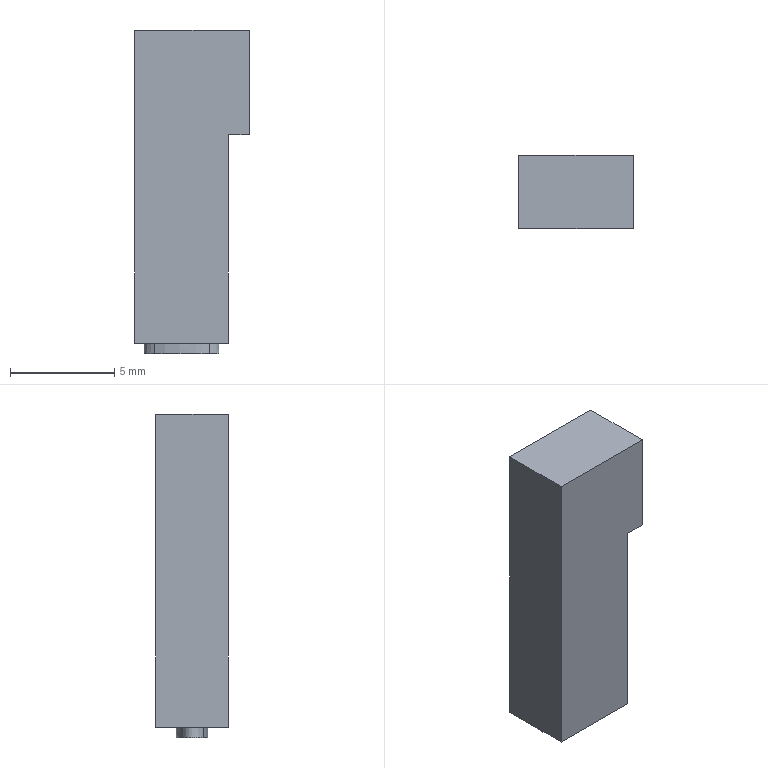Part | STEP file | gslz 2016.10.28-10_id1658_x_t | 1 solid | 15 faces | box 5.5 x 3.5 x 15.5 mm | volume 254.67 mm3 | plane 10 | other 5
STEP:
#1=CARTESIAN_POINT('',(0.,0.,0.));
#2=DIRECTION('',(0.,0.,1.));
#3=DIRECTION('',(1.,0.,0.));
#4=AXIS2_PLACEMENT_3D('',#1,#2,#3);
#5=CARTESIAN_POINT('',(-690.499,76.038,0.));
#6=VERTEX_POINT('',#5);
#7=CARTESIAN_POINT('',(-693.11,74.96,0.));
#8=VERTEX_POINT('',#7);
#9=CARTESIAN_POINT('',(-690.499,76.038,0.));
#10=CARTESIAN_POINT('',(-690.821,76.179,0.));
#11=CARTESIAN_POINT('',(-691.26,76.249,0.));
#12=CARTESIAN_POINT('',(-692.38,76.249,0.));
#13=CARTESIAN_POINT('',(-692.816,76.179,0.));
#14=CARTESIAN_POINT('',(-693.444,75.897,0.));
#15=CARTESIAN_POINT('',(-693.601,75.72,0.));
#16=CARTESIAN_POINT('',(-693.601,75.283,0.));
#17=CARTESIAN_POINT('',(-693.437,75.101,0.));
#18=CARTESIAN_POINT('',(-693.11,74.96,0.));
#19=B_SPLINE_CURVE_WITH_KNOTS('',3,(#9,#10,#11,#12,#13,#14,#15,#16,#17,#18),.UNSPECIFIED.,.F.,.F.,(4,2,2,2,4),(0.,0.2476,0.4947,0.7418,1.),.UNSPECIFIED.);
#20=CARTESIAN_POINT('',(-694.06,75.499,0.));
#21=DIRECTION('',(0.,0.,1.));
#22=DIRECTION('',(1.,0.,0.));
#23=AXIS2_PLACEMENT_3D('',#20,#21,#22);
#24=PLANE('',#23);
#25=CARTESIAN_POINT('',(3.561,0.539));
#26=CARTESIAN_POINT('',(3.239,0.6797));
#27=CARTESIAN_POINT('',(2.8,0.75));
#28=CARTESIAN_POINT('',(1.68,0.75));
#29=CARTESIAN_POINT('',(1.244,0.6797));
#30=CARTESIAN_POINT('',(0.6161,0.3984));
#31=CARTESIAN_POINT('',(0.4587,0.2209));
#32=CARTESIAN_POINT('',(0.4587,-0.2161));
#33=CARTESIAN_POINT('',(0.6228,-0.3977));
#34=CARTESIAN_POINT('',(0.95,-0.539));
#35=B_SPLINE_CURVE_WITH_KNOTS('',3,(#25,#26,#27,#28,#29,#30,#31,#32,#33,#34),.UNSPECIFIED.,.F.,.F.,(4,2,2,2,4),(0.,0.2476,0.4947,0.7418,1.),.UNSPECIFIED.);
#36=(GEOMETRIC_REPRESENTATION_CONTEXT(2)PARAMETRIC_REPRESENTATION_CONTEXT()REPRESENTATION_CONTEXT('',''));
#37=DEFINITIONAL_REPRESENTATION('',(#35),#36);
#38=PCURVE('',#24,#37);
#39=CARTESIAN_POINT('',(-693.11,74.96,-0.5));
#40=CARTESIAN_POINT('',(-693.437,75.101,-0.5));
#41=CARTESIAN_POINT('',(-693.601,75.283,-0.5));
#42=CARTESIAN_POINT('',(-693.601,75.72,-0.5));
#43=CARTESIAN_POINT('',(-693.444,75.897,-0.5));
#44=CARTESIAN_POINT('',(-692.816,76.179,-0.5));
#45=CARTESIAN_POINT('',(-692.38,76.249,-0.5));
#46=CARTESIAN_POINT('',(-691.26,76.249,-0.5));
#47=CARTESIAN_POINT('',(-690.821,76.179,-0.5));
#48=CARTESIAN_POINT('',(-690.499,76.038,-0.5));
#49=B_SPLINE_CURVE_WITH_KNOTS('',3,(#39,#40,#41,#42,#43,#44,#45,#46,#47,#48),.UNSPECIFIED.,.F.,.F.,(4,2,2,2,4),(0.,0.2582,0.5053,0.7524,1.),.UNSPECIFIED.);
#50=DIRECTION('',(0.,0.,1.));
#51=VECTOR('',#50,1.);
#52=SURFACE_OF_LINEAR_EXTRUSION('',#49,#51);
#53=CARTESIAN_POINT('',(1.,0.5));
#54=DIRECTION('',(-1.,0.));
#55=VECTOR('',#54,1.);
#56=LINE('',#53,#55);
#57=(GEOMETRIC_REPRESENTATION_CONTEXT(2)PARAMETRIC_REPRESENTATION_CONTEXT()REPRESENTATION_CONTEXT('',''));
#58=DEFINITIONAL_REPRESENTATION('',(#56),#57);
#59=PCURVE('',#52,#58);
#60=SURFACE_CURVE('',#19,(#38,#59),.PCURVE_S1.);
#61=EDGE_CURVE('',#6,#8,#60,.T.);
#62=ORIENTED_EDGE('',*,*,#61,.T.);
#63=CARTESIAN_POINT('',(-690.49,74.967,0.));
#64=VERTEX_POINT('',#63);
#65=CARTESIAN_POINT('',(-693.11,74.96,0.));
#66=CARTESIAN_POINT('',(-692.782,74.819,0.));
#67=CARTESIAN_POINT('',(-692.352,74.749,0.));
#68=CARTESIAN_POINT('',(-691.247,74.749,0.));
#69=CARTESIAN_POINT('',(-690.804,74.822,0.));
#70=CARTESIAN_POINT('',(-690.49,74.967,0.));
#71=B_SPLINE_CURVE_WITH_KNOTS('',3,(#65,#66,#67,#68,#69,#70),.UNSPECIFIED.,.F.,.F.,(4,2,4),(0.,0.4809,1.),.UNSPECIFIED.);
#72=CARTESIAN_POINT('',(0.95,-0.539));
#73=CARTESIAN_POINT('',(1.278,-0.6797));
#74=CARTESIAN_POINT('',(1.708,-0.75));
#75=CARTESIAN_POINT('',(2.813,-0.75));
#76=CARTESIAN_POINT('',(3.256,-0.6769));
#77=CARTESIAN_POINT('',(3.57,-0.5315));
#78=B_SPLINE_CURVE_WITH_KNOTS('',3,(#72,#73,#74,#75,#76,#77),.UNSPECIFIED.,.F.,.F.,(4,2,4),(0.,0.4809,1.),.UNSPECIFIED.);
#79=(GEOMETRIC_REPRESENTATION_CONTEXT(2)PARAMETRIC_REPRESENTATION_CONTEXT()REPRESENTATION_CONTEXT('',''));
#80=DEFINITIONAL_REPRESENTATION('',(#78),#79);
#81=PCURVE('',#24,#80);
#82=CARTESIAN_POINT('',(-690.49,74.967,-0.5));
#83=CARTESIAN_POINT('',(-690.804,74.822,-0.5));
#84=CARTESIAN_POINT('',(-691.247,74.749,-0.5));
#85=CARTESIAN_POINT('',(-692.352,74.749,-0.5));
#86=CARTESIAN_POINT('',(-692.782,74.819,-0.5));
#87=CARTESIAN_POINT('',(-693.11,74.96,-0.5));
#88=B_SPLINE_CURVE_WITH_KNOTS('',3,(#82,#83,#84,#85,#86,#87),.UNSPECIFIED.,.F.,.F.,(4,2,4),(0.,0.5191,1.),.UNSPECIFIED.);
#89=DIRECTION('',(0.,0.,1.));
#90=VECTOR('',#89,1.);
#91=SURFACE_OF_LINEAR_EXTRUSION('',#88,#90);
#92=CARTESIAN_POINT('',(1.,0.5));
#93=DIRECTION('',(-1.,0.));
#94=VECTOR('',#93,1.);
#95=LINE('',#92,#94);
#96=(GEOMETRIC_REPRESENTATION_CONTEXT(2)PARAMETRIC_REPRESENTATION_CONTEXT()REPRESENTATION_CONTEXT('',''));
#97=DEFINITIONAL_REPRESENTATION('',(#95),#96);
#98=PCURVE('',#91,#97);
#99=SURFACE_CURVE('',#71,(#81,#98),.PCURVE_S1.);
#100=EDGE_CURVE('',#8,#64,#99,.T.);
#101=ORIENTED_EDGE('',*,*,#100,.T.);
#102=CARTESIAN_POINT('',(-690.49,74.967,0.));
#103=CARTESIAN_POINT('',(-690.175,75.113,0.));
#104=CARTESIAN_POINT('',(-690.019,75.292,0.));
#105=CARTESIAN_POINT('',(-690.019,75.72,0.));
#106=CARTESIAN_POINT('',(-690.179,75.897,0.));
#107=CARTESIAN_POINT('',(-690.499,76.038,0.));
#108=B_SPLINE_CURVE_WITH_KNOTS('',3,(#102,#103,#104,#105,#106,#107),.UNSPECIFIED.,.F.,.F.,(4,2,4),(0.,0.5,1.),.UNSPECIFIED.);
#109=CARTESIAN_POINT('',(3.57,-0.5315));
#110=CARTESIAN_POINT('',(3.885,-0.3861));
#111=CARTESIAN_POINT('',(4.041,-0.2065));
#112=CARTESIAN_POINT('',(4.041,0.2209));
#113=CARTESIAN_POINT('',(3.881,0.3984));
#114=CARTESIAN_POINT('',(3.561,0.539));
#115=B_SPLINE_CURVE_WITH_KNOTS('',3,(#109,#110,#111,#112,#113,#114),.UNSPECIFIED.,.F.,.F.,(4,2,4),(0.,0.5,1.),.UNSPECIFIED.);
#116=(GEOMETRIC_REPRESENTATION_CONTEXT(2)PARAMETRIC_REPRESENTATION_CONTEXT()REPRESENTATION_CONTEXT('',''));
#117=DEFINITIONAL_REPRESENTATION('',(#115),#116);
#118=PCURVE('',#24,#117);
#119=CARTESIAN_POINT('',(-690.499,76.038,-0.5));
#120=CARTESIAN_POINT('',(-690.179,75.897,-0.5));
#121=CARTESIAN_POINT('',(-690.019,75.72,-0.5));
#122=CARTESIAN_POINT('',(-690.019,75.292,-0.5));
#123=CARTESIAN_POINT('',(-690.175,75.113,-0.5));
#124=CARTESIAN_POINT('',(-690.49,74.967,-0.5));
#125=B_SPLINE_CURVE_WITH_KNOTS('',3,(#119,#120,#121,#122,#123,#124),.UNSPECIFIED.,.F.,.F.,(4,2,4),(0.,0.5,1.),.UNSPECIFIED.);
#126=DIRECTION('',(0.,0.,1.));
#127=VECTOR('',#126,1.);
#128=SURFACE_OF_LINEAR_EXTRUSION('',#125,#127);
#129=CARTESIAN_POINT('',(1.,0.5));
#130=DIRECTION('',(-1.,0.));
#131=VECTOR('',#130,1.);
#132=LINE('',#129,#131);
#133=(GEOMETRIC_REPRESENTATION_CONTEXT(2)PARAMETRIC_REPRESENTATION_CONTEXT()REPRESENTATION_CONTEXT('',''));
#134=DEFINITIONAL_REPRESENTATION('',(#132),#133);
#135=PCURVE('',#128,#134);
#136=SURFACE_CURVE('',#108,(#118,#135),.PCURVE_S1.);
#137=EDGE_CURVE('',#64,#6,#136,.T.);
#138=ORIENTED_EDGE('',*,*,#137,.T.);
#139=EDGE_LOOP('',(#62,#101,#138));
#140=FACE_BOUND('',#139,.T.);
#141=CARTESIAN_POINT('',(-689.56,77.249,0.));
#142=VERTEX_POINT('',#141);
#143=CARTESIAN_POINT('',(-689.56,73.749,0.));
#144=VERTEX_POINT('',#143);
#145=CARTESIAN_POINT('',(-689.56,75.499,0.));
#146=DIRECTION('',(0.,-1.,0.));
#147=VECTOR('',#146,1.);
#148=LINE('',#145,#147);
#149=CARTESIAN_POINT('',(4.5,0.));
#150=DIRECTION('',(0.,-1.));
#151=VECTOR('',#150,1.);
#152=LINE('',#149,#151);
#153=(GEOMETRIC_REPRESENTATION_CONTEXT(2)PARAMETRIC_REPRESENTATION_CONTEXT()REPRESENTATION_CONTEXT('',''));
#154=DEFINITIONAL_REPRESENTATION('',(#152),#153);
#155=PCURVE('',#24,#154);
#156=CARTESIAN_POINT('',(-689.56,75.499,7.5));
#157=DIRECTION('',(1.,0.,0.));
#158=DIRECTION('',(0.,0.,-1.));
#159=AXIS2_PLACEMENT_3D('',#156,#157,#158);
#160=PLANE('',#159);
#161=CARTESIAN_POINT('',(7.5,0.000000303));
#162=DIRECTION('',(0.,-1.));
#163=VECTOR('',#162,1.);
#164=LINE('',#161,#163);
#165=(GEOMETRIC_REPRESENTATION_CONTEXT(2)PARAMETRIC_REPRESENTATION_CONTEXT()REPRESENTATION_CONTEXT('',''));
#166=DEFINITIONAL_REPRESENTATION('',(#164),#165);
#167=PCURVE('',#160,#166);
#168=SURFACE_CURVE('',#148,(#155,#167),.PCURVE_S1.);
#169=EDGE_CURVE('',#142,#144,#168,.T.);
#170=ORIENTED_EDGE('',*,*,#169,.T.);
#171=CARTESIAN_POINT('',(-694.06,73.749,0.));
#172=VERTEX_POINT('',#171);
#173=CARTESIAN_POINT('',(-691.31,73.749,0.));
#174=DIRECTION('',(-1.,0.000000055,0.));
#175=VECTOR('',#174,1.);
#176=LINE('',#173,#175);
#177=CARTESIAN_POINT('',(2.75,-1.75));
#178=DIRECTION('',(-1.,0.000000055));
#179=VECTOR('',#178,1.);
#180=LINE('',#177,#179);
#181=(GEOMETRIC_REPRESENTATION_CONTEXT(2)PARAMETRIC_REPRESENTATION_CONTEXT()REPRESENTATION_CONTEXT('',''));
#182=DEFINITIONAL_REPRESENTATION('',(#180),#181);
#183=PCURVE('',#24,#182);
#184=CARTESIAN_POINT('',(-694.06,73.749,15.));
#185=DIRECTION('',(-0.000000055,-1.,0.));
#186=DIRECTION('',(-1.,0.000000055,0.));
#187=AXIS2_PLACEMENT_3D('',#184,#185,#186);
#188=PLANE('',#187);
#189=CARTESIAN_POINT('',(-2.75,15.));
#190=DIRECTION('',(1.,0.));
#191=VECTOR('',#190,1.);
#192=LINE('',#189,#191);
#193=(GEOMETRIC_REPRESENTATION_CONTEXT(2)PARAMETRIC_REPRESENTATION_CONTEXT()REPRESENTATION_CONTEXT('',''));
#194=DEFINITIONAL_REPRESENTATION('',(#192),#193);
#195=PCURVE('',#188,#194);
#196=SURFACE_CURVE('',#176,(#183,#195),.PCURVE_S1.);
#197=EDGE_CURVE('',#144,#172,#196,.T.);
#198=ORIENTED_EDGE('',*,*,#197,.T.);
#199=CARTESIAN_POINT('',(-694.06,77.249,0.));
#200=VERTEX_POINT('',#199);
#201=CARTESIAN_POINT('',(-694.06,75.499,0.));
#202=DIRECTION('',(0.,1.,0.));
#203=VECTOR('',#202,1.);
#204=LINE('',#201,#203);
#205=CARTESIAN_POINT('',(0.,0.));
#206=DIRECTION('',(0.,1.));
#207=VECTOR('',#206,1.);
#208=LINE('',#205,#207);
#209=(GEOMETRIC_REPRESENTATION_CONTEXT(2)PARAMETRIC_REPRESENTATION_CONTEXT()REPRESENTATION_CONTEXT('',''));
#210=DEFINITIONAL_REPRESENTATION('',(#208),#209);
#211=PCURVE('',#24,#210);
#212=CARTESIAN_POINT('',(-694.06,77.249,15.));
#213=DIRECTION('',(-1.,0.,0.));
#214=DIRECTION('',(0.,1.,0.));
#215=AXIS2_PLACEMENT_3D('',#212,#213,#214);
#216=PLANE('',#215);
#217=CARTESIAN_POINT('',(-1.75,15.));
#218=DIRECTION('',(1.,0.));
#219=VECTOR('',#218,1.);
#220=LINE('',#217,#219);
#221=(GEOMETRIC_REPRESENTATION_CONTEXT(2)PARAMETRIC_REPRESENTATION_CONTEXT()REPRESENTATION_CONTEXT('',''));
#222=DEFINITIONAL_REPRESENTATION('',(#220),#221);
#223=PCURVE('',#216,#222);
#224=SURFACE_CURVE('',#204,(#211,#223),.PCURVE_S1.);
#225=EDGE_CURVE('',#172,#200,#224,.T.);
#226=ORIENTED_EDGE('',*,*,#225,.T.);
#227=CARTESIAN_POINT('',(-691.31,77.249,0.));
#228=DIRECTION('',(1.,-0.000000055,0.));
#229=VECTOR('',#228,1.);
#230=LINE('',#227,#229);
#231=CARTESIAN_POINT('',(2.75,1.75));
#232=DIRECTION('',(1.,-0.000000055));
#233=VECTOR('',#232,1.);
#234=LINE('',#231,#233);
#235=(GEOMETRIC_REPRESENTATION_CONTEXT(2)PARAMETRIC_REPRESENTATION_CONTEXT()REPRESENTATION_CONTEXT('',''));
#236=DEFINITIONAL_REPRESENTATION('',(#234),#235);
#237=PCURVE('',#24,#236);
#238=CARTESIAN_POINT('',(-688.56,77.249,15.));
#239=DIRECTION('',(0.000000055,1.,0.));
#240=DIRECTION('',(1.,-0.000000055,0.));
#241=AXIS2_PLACEMENT_3D('',#238,#239,#240);
#242=PLANE('',#241);
#243=CARTESIAN_POINT('',(-2.75,15.));
#244=DIRECTION('',(1.,0.));
#245=VECTOR('',#244,1.);
#246=LINE('',#243,#245);
#247=(GEOMETRIC_REPRESENTATION_CONTEXT(2)PARAMETRIC_REPRESENTATION_CONTEXT()REPRESENTATION_CONTEXT('',''));
#248=DEFINITIONAL_REPRESENTATION('',(#246),#247);
#249=PCURVE('',#242,#248);
#250=SURFACE_CURVE('',#230,(#237,#249),.PCURVE_S1.);
#251=EDGE_CURVE('',#200,#142,#250,.T.);
#252=ORIENTED_EDGE('',*,*,#251,.T.);
#253=EDGE_LOOP('',(#170,#198,#226,#252));
#254=FACE_BOUND('',#253,.T.);
#255=ADVANCED_FACE('',(#140,#254),#24,.F.);
#256=CARTESIAN_POINT('',(-688.56,73.749,15.));
#257=VERTEX_POINT('',#256);
#258=CARTESIAN_POINT('',(-694.06,73.749,15.));
#259=VERTEX_POINT('',#258);
#260=CARTESIAN_POINT('',(-691.31,73.749,15.));
#261=DIRECTION('',(-1.,0.000000055,0.));
#262=VECTOR('',#261,1.);
#263=LINE('',#260,#262);
#264=CARTESIAN_POINT('',(-2.75,0.));
#265=DIRECTION('',(1.,0.));
#266=VECTOR('',#265,1.);
#267=LINE('',#264,#266);
#268=(GEOMETRIC_REPRESENTATION_CONTEXT(2)PARAMETRIC_REPRESENTATION_CONTEXT()REPRESENTATION_CONTEXT('',''));
#269=DEFINITIONAL_REPRESENTATION('',(#267),#268);
#270=PCURVE('',#188,#269);
#271=CARTESIAN_POINT('',(-694.06,75.499,15.));
#272=DIRECTION('',(0.,0.,1.));
#273=DIRECTION('',(1.,0.,0.));
#274=AXIS2_PLACEMENT_3D('',#271,#272,#273);
#275=PLANE('',#274);
#276=CARTESIAN_POINT('',(2.75,-1.75));
#277=DIRECTION('',(-1.,0.000000055));
#278=VECTOR('',#277,1.);
#279=LINE('',#276,#278);
#280=(GEOMETRIC_REPRESENTATION_CONTEXT(2)PARAMETRIC_REPRESENTATION_CONTEXT()REPRESENTATION_CONTEXT('',''));
#281=DEFINITIONAL_REPRESENTATION('',(#279),#280);
#282=PCURVE('',#275,#281);
#283=SURFACE_CURVE('',#263,(#270,#282),.PCURVE_S1.);
#284=EDGE_CURVE('',#257,#259,#283,.T.);
#285=ORIENTED_EDGE('',*,*,#284,.T.);
#286=CARTESIAN_POINT('',(-694.06,73.749,15.));
#287=DIRECTION('',(0.,0.,1.));
#288=VECTOR('',#287,1.);
#289=LINE('',#286,#288);
#290=CARTESIAN_POINT('',(0.,0.));
#291=DIRECTION('',(0.,-1.));
#292=VECTOR('',#291,1.);
#293=LINE('',#290,#292);
#294=(GEOMETRIC_REPRESENTATION_CONTEXT(2)PARAMETRIC_REPRESENTATION_CONTEXT()REPRESENTATION_CONTEXT('',''));
#295=DEFINITIONAL_REPRESENTATION('',(#293),#294);
#296=PCURVE('',#188,#295);
#297=CARTESIAN_POINT('',(-3.5,0.));
#298=DIRECTION('',(0.,-1.));
#299=VECTOR('',#298,1.);
#300=LINE('',#297,#299);
#301=(GEOMETRIC_REPRESENTATION_CONTEXT(2)PARAMETRIC_REPRESENTATION_CONTEXT()REPRESENTATION_CONTEXT('',''));
#302=DEFINITIONAL_REPRESENTATION('',(#300),#301);
#303=PCURVE('',#216,#302);
#304=SURFACE_CURVE('',#289,(#296,#303),.PCURVE_S1.);
#305=EDGE_CURVE('',#172,#259,#304,.T.);
#306=ORIENTED_EDGE('',*,*,#305,.F.);
#307=ORIENTED_EDGE('',*,*,#197,.F.);
#308=CARTESIAN_POINT('',(-689.56,73.749,10.));
#309=VERTEX_POINT('',#308);
#310=CARTESIAN_POINT('',(-689.56,73.749,15.));
#311=DIRECTION('',(0.,0.,-1.));
#312=VECTOR('',#311,1.);
#313=LINE('',#310,#312);
#314=CARTESIAN_POINT('',(-4.5,0.));
#315=DIRECTION('',(0.,1.));
#316=VECTOR('',#315,1.);
#317=LINE('',#314,#316);
#318=(GEOMETRIC_REPRESENTATION_CONTEXT(2)PARAMETRIC_REPRESENTATION_CONTEXT()REPRESENTATION_CONTEXT('',''));
#319=DEFINITIONAL_REPRESENTATION('',(#317),#318);
#320=PCURVE('',#188,#319);
#321=CARTESIAN_POINT('',(-7.5,-1.75));
#322=DIRECTION('',(1.,0.));
#323=VECTOR('',#322,1.);
#324=LINE('',#321,#323);
#325=(GEOMETRIC_REPRESENTATION_CONTEXT(2)PARAMETRIC_REPRESENTATION_CONTEXT()REPRESENTATION_CONTEXT('',''));
#326=DEFINITIONAL_REPRESENTATION('',(#324),#325);
#327=PCURVE('',#160,#326);
#328=SURFACE_CURVE('',#313,(#320,#327),.PCURVE_S1.);
#329=EDGE_CURVE('',#309,#144,#328,.T.);
#330=ORIENTED_EDGE('',*,*,#329,.F.);
#331=CARTESIAN_POINT('',(-688.56,73.749,10.));
#332=VERTEX_POINT('',#331);
#333=CARTESIAN_POINT('',(-694.06,73.749,10.));
#334=DIRECTION('',(-1.,0.000000055,0.));
#335=VECTOR('',#334,1.);
#336=LINE('',#333,#335);
#337=CARTESIAN_POINT('',(0.,5.));
#338=DIRECTION('',(1.,0.));
#339=VECTOR('',#338,1.);
#340=LINE('',#337,#339);
#341=(GEOMETRIC_REPRESENTATION_CONTEXT(2)PARAMETRIC_REPRESENTATION_CONTEXT()REPRESENTATION_CONTEXT('',''));
#342=DEFINITIONAL_REPRESENTATION('',(#340),#341);
#343=PCURVE('',#188,#342);
#344=CARTESIAN_POINT('',(-694.06,75.499,10.));
#345=DIRECTION('',(0.,0.,1.));
#346=DIRECTION('',(1.,0.,0.));
#347=AXIS2_PLACEMENT_3D('',#344,#345,#346);
#348=PLANE('',#347);
#349=CARTESIAN_POINT('',(0.,-1.75));
#350=DIRECTION('',(-1.,0.000000055));
#351=VECTOR('',#350,1.);
#352=LINE('',#349,#351);
#353=(GEOMETRIC_REPRESENTATION_CONTEXT(2)PARAMETRIC_REPRESENTATION_CONTEXT()REPRESENTATION_CONTEXT('',''));
#354=DEFINITIONAL_REPRESENTATION('',(#352),#353);
#355=PCURVE('',#348,#354);
#356=SURFACE_CURVE('',#336,(#343,#355),.PCURVE_S1.);
#357=EDGE_CURVE('',#332,#309,#356,.T.);
#358=ORIENTED_EDGE('',*,*,#357,.F.);
#359=CARTESIAN_POINT('',(-688.56,73.749,15.));
#360=DIRECTION('',(0.,0.,1.));
#361=VECTOR('',#360,1.);
#362=LINE('',#359,#361);
#363=CARTESIAN_POINT('',(-5.5,0.));
#364=DIRECTION('',(0.,-1.));
#365=VECTOR('',#364,1.);
#366=LINE('',#363,#365);
#367=(GEOMETRIC_REPRESENTATION_CONTEXT(2)PARAMETRIC_REPRESENTATION_CONTEXT()REPRESENTATION_CONTEXT('',''));
#368=DEFINITIONAL_REPRESENTATION('',(#366),#367);
#369=PCURVE('',#188,#368);
#370=CARTESIAN_POINT('',(-688.56,73.749,15.));
#371=DIRECTION('',(1.,0.,0.));
#372=DIRECTION('',(0.,-1.,0.));
#373=AXIS2_PLACEMENT_3D('',#370,#371,#372);
#374=PLANE('',#373);
#375=CARTESIAN_POINT('',(0.,0.));
#376=DIRECTION('',(0.,-1.));
#377=VECTOR('',#376,1.);
#378=LINE('',#375,#377);
#379=(GEOMETRIC_REPRESENTATION_CONTEXT(2)PARAMETRIC_REPRESENTATION_CONTEXT()REPRESENTATION_CONTEXT('',''));
#380=DEFINITIONAL_REPRESENTATION('',(#378),#379);
#381=PCURVE('',#374,#380);
#382=SURFACE_CURVE('',#362,(#369,#381),.PCURVE_S1.);
#383=EDGE_CURVE('',#332,#257,#382,.T.);
#384=ORIENTED_EDGE('',*,*,#383,.T.);
#385=EDGE_LOOP('',(#285,#306,#307,#330,#358,#384));
#386=FACE_BOUND('',#385,.T.);
#387=ADVANCED_FACE('',(#386),#188,.T.);
#388=ORIENTED_EDGE('',*,*,#251,.F.);
#389=CARTESIAN_POINT('',(-694.06,77.249,15.));
#390=VERTEX_POINT('',#389);
#391=CARTESIAN_POINT('',(-694.06,77.249,15.));
#392=DIRECTION('',(0.,0.,1.));
#393=VECTOR('',#392,1.);
#394=LINE('',#391,#393);
#395=CARTESIAN_POINT('',(-5.5,0.));
#396=DIRECTION('',(0.,-1.));
#397=VECTOR('',#396,1.);
#398=LINE('',#395,#397);
#399=(GEOMETRIC_REPRESENTATION_CONTEXT(2)PARAMETRIC_REPRESENTATION_CONTEXT()REPRESENTATION_CONTEXT('',''));
#400=DEFINITIONAL_REPRESENTATION('',(#398),#399);
#401=PCURVE('',#242,#400);
#402=CARTESIAN_POINT('',(0.,0.));
#403=DIRECTION('',(0.,-1.));
#404=VECTOR('',#403,1.);
#405=LINE('',#402,#404);
#406=(GEOMETRIC_REPRESENTATION_CONTEXT(2)PARAMETRIC_REPRESENTATION_CONTEXT()REPRESENTATION_CONTEXT('',''));
#407=DEFINITIONAL_REPRESENTATION('',(#405),#406);
#408=PCURVE('',#216,#407);
#409=SURFACE_CURVE('',#394,(#401,#408),.PCURVE_S1.);
#410=EDGE_CURVE('',#200,#390,#409,.T.);
#411=ORIENTED_EDGE('',*,*,#410,.T.);
#412=CARTESIAN_POINT('',(-688.56,77.249,15.));
#413=VERTEX_POINT('',#412);
#414=CARTESIAN_POINT('',(-691.31,77.249,15.));
#415=DIRECTION('',(1.,-0.000000055,0.));
#416=VECTOR('',#415,1.);
#417=LINE('',#414,#416);
#418=CARTESIAN_POINT('',(-2.75,0.));
#419=DIRECTION('',(1.,0.));
#420=VECTOR('',#419,1.);
#421=LINE('',#418,#420);
#422=(GEOMETRIC_REPRESENTATION_CONTEXT(2)PARAMETRIC_REPRESENTATION_CONTEXT()REPRESENTATION_CONTEXT('',''));
#423=DEFINITIONAL_REPRESENTATION('',(#421),#422);
#424=PCURVE('',#242,#423);
#425=CARTESIAN_POINT('',(2.75,1.75));
#426=DIRECTION('',(1.,-0.000000055));
#427=VECTOR('',#426,1.);
#428=LINE('',#425,#427);
#429=(GEOMETRIC_REPRESENTATION_CONTEXT(2)PARAMETRIC_REPRESENTATION_CONTEXT()REPRESENTATION_CONTEXT('',''));
#430=DEFINITIONAL_REPRESENTATION('',(#428),#429);
#431=PCURVE('',#275,#430);
#432=SURFACE_CURVE('',#417,(#424,#431),.PCURVE_S1.);
#433=EDGE_CURVE('',#390,#413,#432,.T.);
#434=ORIENTED_EDGE('',*,*,#433,.T.);
#435=CARTESIAN_POINT('',(-688.56,77.249,10.));
#436=VERTEX_POINT('',#435);
#437=CARTESIAN_POINT('',(-688.56,77.249,15.));
#438=DIRECTION('',(0.,0.,1.));
#439=VECTOR('',#438,1.);
#440=LINE('',#437,#439);
#441=CARTESIAN_POINT('',(0.,0.));
#442=DIRECTION('',(0.,-1.));
#443=VECTOR('',#442,1.);
#444=LINE('',#441,#443);
#445=(GEOMETRIC_REPRESENTATION_CONTEXT(2)PARAMETRIC_REPRESENTATION_CONTEXT()REPRESENTATION_CONTEXT('',''));
#446=DEFINITIONAL_REPRESENTATION('',(#444),#445);
#447=PCURVE('',#242,#446);
#448=CARTESIAN_POINT('',(-3.5,0.));
#449=DIRECTION('',(0.,-1.));
#450=VECTOR('',#449,1.);
#451=LINE('',#448,#450);
#452=(GEOMETRIC_REPRESENTATION_CONTEXT(2)PARAMETRIC_REPRESENTATION_CONTEXT()REPRESENTATION_CONTEXT('',''));
#453=DEFINITIONAL_REPRESENTATION('',(#451),#452);
#454=PCURVE('',#374,#453);
#455=SURFACE_CURVE('',#440,(#447,#454),.PCURVE_S1.);
#456=EDGE_CURVE('',#436,#413,#455,.T.);
#457=ORIENTED_EDGE('',*,*,#456,.F.);
#458=CARTESIAN_POINT('',(-689.56,77.249,10.));
#459=VERTEX_POINT('',#458);
#460=CARTESIAN_POINT('',(-688.56,77.249,10.));
#461=DIRECTION('',(1.,-0.000000055,0.));
#462=VECTOR('',#461,1.);
#463=LINE('',#460,#462);
#464=CARTESIAN_POINT('',(0.,5.));
#465=DIRECTION('',(1.,0.));
#466=VECTOR('',#465,1.);
#467=LINE('',#464,#466);
#468=(GEOMETRIC_REPRESENTATION_CONTEXT(2)PARAMETRIC_REPRESENTATION_CONTEXT()REPRESENTATION_CONTEXT('',''));
#469=DEFINITIONAL_REPRESENTATION('',(#467),#468);
#470=PCURVE('',#242,#469);
#471=CARTESIAN_POINT('',(5.5,1.75));
#472=DIRECTION('',(1.,-0.000000055));
#473=VECTOR('',#472,1.);
#474=LINE('',#471,#473);
#475=(GEOMETRIC_REPRESENTATION_CONTEXT(2)PARAMETRIC_REPRESENTATION_CONTEXT()REPRESENTATION_CONTEXT('',''));
#476=DEFINITIONAL_REPRESENTATION('',(#474),#475);
#477=PCURVE('',#348,#476);
#478=SURFACE_CURVE('',#463,(#470,#477),.PCURVE_S1.);
#479=EDGE_CURVE('',#459,#436,#478,.T.);
#480=ORIENTED_EDGE('',*,*,#479,.F.);
#481=CARTESIAN_POINT('',(-689.56,77.249,15.));
#482=DIRECTION('',(0.,0.,1.));
#483=VECTOR('',#482,1.);
#484=LINE('',#481,#483);
#485=CARTESIAN_POINT('',(-1.,0.));
#486=DIRECTION('',(0.,-1.));
#487=VECTOR('',#486,1.);
#488=LINE('',#485,#487);
#489=(GEOMETRIC_REPRESENTATION_CONTEXT(2)PARAMETRIC_REPRESENTATION_CONTEXT()REPRESENTATION_CONTEXT('',''));
#490=DEFINITIONAL_REPRESENTATION('',(#488),#489);
#491=PCURVE('',#242,#490);
#492=CARTESIAN_POINT('',(-7.5,1.75));
#493=DIRECTION('',(-1.,0.));
#494=VECTOR('',#493,1.);
#495=LINE('',#492,#494);
#496=(GEOMETRIC_REPRESENTATION_CONTEXT(2)PARAMETRIC_REPRESENTATION_CONTEXT()REPRESENTATION_CONTEXT('',''));
#497=DEFINITIONAL_REPRESENTATION('',(#495),#496);
#498=PCURVE('',#160,#497);
#499=SURFACE_CURVE('',#484,(#491,#498),.PCURVE_S1.);
#500=EDGE_CURVE('',#142,#459,#499,.T.);
#501=ORIENTED_EDGE('',*,*,#500,.F.);
#502=EDGE_LOOP('',(#388,#411,#434,#457,#480,#501));
#503=FACE_BOUND('',#502,.T.);
#504=ADVANCED_FACE('',(#503),#242,.T.);
#505=ORIENTED_EDGE('',*,*,#433,.F.);
#506=CARTESIAN_POINT('',(-694.06,75.499,15.));
#507=DIRECTION('',(0.,1.,0.));
#508=VECTOR('',#507,1.);
#509=LINE('',#506,#508);
#510=CARTESIAN_POINT('',(0.,0.));
#511=DIRECTION('',(0.,1.));
#512=VECTOR('',#511,1.);
#513=LINE('',#510,#512);
#514=(GEOMETRIC_REPRESENTATION_CONTEXT(2)PARAMETRIC_REPRESENTATION_CONTEXT()REPRESENTATION_CONTEXT('',''));
#515=DEFINITIONAL_REPRESENTATION('',(#513),#514);
#516=PCURVE('',#275,#515);
#517=CARTESIAN_POINT('',(-1.75,0.));
#518=DIRECTION('',(1.,0.));
#519=VECTOR('',#518,1.);
#520=LINE('',#517,#519);
#521=(GEOMETRIC_REPRESENTATION_CONTEXT(2)PARAMETRIC_REPRESENTATION_CONTEXT()REPRESENTATION_CONTEXT('',''));
#522=DEFINITIONAL_REPRESENTATION('',(#520),#521);
#523=PCURVE('',#216,#522);
#524=SURFACE_CURVE('',#509,(#516,#523),.PCURVE_S1.);
#525=EDGE_CURVE('',#259,#390,#524,.T.);
#526=ORIENTED_EDGE('',*,*,#525,.F.);
#527=ORIENTED_EDGE('',*,*,#284,.F.);
#528=CARTESIAN_POINT('',(-688.56,75.499,15.));
#529=DIRECTION('',(0.,-1.,0.));
#530=VECTOR('',#529,1.);
#531=LINE('',#528,#530);
#532=CARTESIAN_POINT('',(5.5,-0.000000303));
#533=DIRECTION('',(0.,-1.));
#534=VECTOR('',#533,1.);
#535=LINE('',#532,#534);
#536=(GEOMETRIC_REPRESENTATION_CONTEXT(2)PARAMETRIC_REPRESENTATION_CONTEXT()REPRESENTATION_CONTEXT('',''));
#537=DEFINITIONAL_REPRESENTATION('',(#535),#536);
#538=PCURVE('',#275,#537);
#539=CARTESIAN_POINT('',(-1.75,0.));
#540=DIRECTION('',(1.,0.));
#541=VECTOR('',#540,1.);
#542=LINE('',#539,#541);
#543=(GEOMETRIC_REPRESENTATION_CONTEXT(2)PARAMETRIC_REPRESENTATION_CONTEXT()REPRESENTATION_CONTEXT('',''));
#544=DEFINITIONAL_REPRESENTATION('',(#542),#543);
#545=PCURVE('',#374,#544);
#546=SURFACE_CURVE('',#531,(#538,#545),.PCURVE_S1.);
#547=EDGE_CURVE('',#413,#257,#546,.T.);
#548=ORIENTED_EDGE('',*,*,#547,.F.);
#549=EDGE_LOOP('',(#505,#526,#527,#548));
#550=FACE_BOUND('',#549,.T.);
#551=ADVANCED_FACE('',(#550),#275,.T.);
#552=ORIENTED_EDGE('',*,*,#225,.F.);
#553=ORIENTED_EDGE('',*,*,#305,.T.);
#554=ORIENTED_EDGE('',*,*,#525,.T.);
#555=ORIENTED_EDGE('',*,*,#410,.F.);
#556=EDGE_LOOP('',(#552,#553,#554,#555));
#557=FACE_BOUND('',#556,.T.);
#558=ADVANCED_FACE('',(#557),#216,.T.);
#559=CARTESIAN_POINT('',(-689.56,75.499,10.));
#560=DIRECTION('',(0.,1.,0.));
#561=VECTOR('',#560,1.);
#562=LINE('',#559,#561);
#563=CARTESIAN_POINT('',(-2.5,0.000000303));
#564=DIRECTION('',(0.,1.));
#565=VECTOR('',#564,1.);
#566=LINE('',#563,#565);
#567=(GEOMETRIC_REPRESENTATION_CONTEXT(2)PARAMETRIC_REPRESENTATION_CONTEXT()REPRESENTATION_CONTEXT('',''));
#568=DEFINITIONAL_REPRESENTATION('',(#566),#567);
#569=PCURVE('',#160,#568);
#570=CARTESIAN_POINT('',(4.5,0.));
#571=DIRECTION('',(0.,1.));
#572=VECTOR('',#571,1.);
#573=LINE('',#570,#572);
#574=(GEOMETRIC_REPRESENTATION_CONTEXT(2)PARAMETRIC_REPRESENTATION_CONTEXT()REPRESENTATION_CONTEXT('',''));
#575=DEFINITIONAL_REPRESENTATION('',(#573),#574);
#576=PCURVE('',#348,#575);
#577=SURFACE_CURVE('',#562,(#569,#576),.PCURVE_S1.);
#578=EDGE_CURVE('',#309,#459,#577,.T.);
#579=ORIENTED_EDGE('',*,*,#578,.F.);
#580=ORIENTED_EDGE('',*,*,#329,.T.);
#581=ORIENTED_EDGE('',*,*,#169,.F.);
#582=ORIENTED_EDGE('',*,*,#500,.T.);
#583=EDGE_LOOP('',(#579,#580,#581,#582));
#584=FACE_BOUND('',#583,.T.);
#585=ADVANCED_FACE('',(#584),#160,.T.);
#586=CARTESIAN_POINT('',(-688.56,73.749,10.));
#587=DIRECTION('',(0.,-1.,0.));
#588=VECTOR('',#587,1.);
#589=LINE('',#586,#588);
#590=CARTESIAN_POINT('',(0.,5.));
#591=DIRECTION('',(1.,0.));
#592=VECTOR('',#591,1.);
#593=LINE('',#590,#592);
#594=(GEOMETRIC_REPRESENTATION_CONTEXT(2)PARAMETRIC_REPRESENTATION_CONTEXT()REPRESENTATION_CONTEXT('',''));
#595=DEFINITIONAL_REPRESENTATION('',(#593),#594);
#596=PCURVE('',#374,#595);
#597=CARTESIAN_POINT('',(5.5,-1.75));
#598=DIRECTION('',(0.,-1.));
#599=VECTOR('',#598,1.);
#600=LINE('',#597,#599);
#601=(GEOMETRIC_REPRESENTATION_CONTEXT(2)PARAMETRIC_REPRESENTATION_CONTEXT()REPRESENTATION_CONTEXT('',''));
#602=DEFINITIONAL_REPRESENTATION('',(#600),#601);
#603=PCURVE('',#348,#602);
#604=SURFACE_CURVE('',#589,(#596,#603),.PCURVE_S1.);
#605=EDGE_CURVE('',#436,#332,#604,.T.);
#606=ORIENTED_EDGE('',*,*,#605,.F.);
#607=ORIENTED_EDGE('',*,*,#456,.T.);
#608=ORIENTED_EDGE('',*,*,#547,.T.);
#609=ORIENTED_EDGE('',*,*,#383,.F.);
#610=EDGE_LOOP('',(#606,#607,#608,#609));
#611=FACE_BOUND('',#610,.T.);
#612=ADVANCED_FACE('',(#611),#374,.T.);
#613=ORIENTED_EDGE('',*,*,#479,.T.);
#614=ORIENTED_EDGE('',*,*,#605,.T.);
#615=ORIENTED_EDGE('',*,*,#357,.T.);
#616=ORIENTED_EDGE('',*,*,#578,.T.);
#617=EDGE_LOOP('',(#613,#614,#615,#616));
#618=FACE_BOUND('',#617,.T.);
#619=ADVANCED_FACE('',(#618),#348,.F.);
#620=CARTESIAN_POINT('',(-692.997,75.856,-0.5));
#621=VERTEX_POINT('',#620);
#622=CARTESIAN_POINT('',(-692.997,75.856,0.));
#623=VERTEX_POINT('',#622);
#624=CARTESIAN_POINT('',(-692.997,75.856,-0.5));
#625=DIRECTION('',(0.,0.,1.));
#626=VECTOR('',#625,1.);
#627=LINE('',#624,#626);
#628=CARTESIAN_POINT('',(-692.997,75.856,-0.5));
#629=CARTESIAN_POINT('',(-693.29,75.779,-0.5));
#630=CARTESIAN_POINT('',(-693.437,75.662,-0.5));
#631=CARTESIAN_POINT('',(-693.437,75.37,-0.5));
#632=CARTESIAN_POINT('',(-693.29,75.256,-0.5));
#633=CARTESIAN_POINT('',(-692.703,75.072,-0.5));
#634=CARTESIAN_POINT('',(-692.312,75.026,-0.5));
#635=CARTESIAN_POINT('',(-691.302,75.026,-0.5));
#636=CARTESIAN_POINT('',(-690.9,75.072,-0.5));
#637=CARTESIAN_POINT('',(-690.613,75.164,-0.5));
#638=B_SPLINE_CURVE_WITH_KNOTS('',3,(#628,#629,#630,#631,#632,#633,#634,#635,#636,#637),.UNSPECIFIED.,.F.,.F.,(4,2,2,2,4),(0.,0.2726,0.5106,0.7486,1.),.UNSPECIFIED.);
#639=DIRECTION('',(0.,0.,1.));
#640=VECTOR('',#639,1.);
#641=SURFACE_OF_LINEAR_EXTRUSION('',#638,#640);
#642=CARTESIAN_POINT('',(0.,0.));
#643=DIRECTION('',(0.,1.));
#644=VECTOR('',#643,1.);
#645=LINE('',#642,#644);
#646=(GEOMETRIC_REPRESENTATION_CONTEXT(2)PARAMETRIC_REPRESENTATION_CONTEXT()REPRESENTATION_CONTEXT('',''));
#647=DEFINITIONAL_REPRESENTATION('',(#645),#646);
#648=PCURVE('',#641,#647);
#649=CARTESIAN_POINT('',(-690.613,75.164,-0.5));
#650=CARTESIAN_POINT('',(-690.326,75.256,-0.5));
#651=CARTESIAN_POINT('',(-690.183,75.37,-0.5));
#652=CARTESIAN_POINT('',(-690.183,75.652,-0.5));
#653=CARTESIAN_POINT('',(-690.326,75.766,-0.5));
#654=CARTESIAN_POINT('',(-690.9,75.932,-0.5));
#655=CARTESIAN_POINT('',(-691.302,75.973,-0.5));
#656=CARTESIAN_POINT('',(-692.312,75.973,-0.5));
#657=CARTESIAN_POINT('',(-692.703,75.934,-0.5));
#658=CARTESIAN_POINT('',(-692.997,75.856,-0.5));
#659=B_SPLINE_CURVE_WITH_KNOTS('',3,(#649,#650,#651,#652,#653,#654,#655,#656,#657,#658),.UNSPECIFIED.,.F.,.F.,(4,2,2,2,4),(0.,0.2399,0.4979,0.7559,1.),.UNSPECIFIED.);
#660=DIRECTION('',(0.,0.,1.));
#661=VECTOR('',#660,1.);
#662=SURFACE_OF_LINEAR_EXTRUSION('',#659,#661);
#663=CARTESIAN_POINT('',(1.,0.));
#664=DIRECTION('',(0.,1.));
#665=VECTOR('',#664,1.);
#666=LINE('',#663,#665);
#667=(GEOMETRIC_REPRESENTATION_CONTEXT(2)PARAMETRIC_REPRESENTATION_CONTEXT()REPRESENTATION_CONTEXT('',''));
#668=DEFINITIONAL_REPRESENTATION('',(#666),#667);
#669=PCURVE('',#662,#668);
#670=SURFACE_CURVE('',#627,(#648,#669),.PCURVE_S1.);
#671=EDGE_CURVE('',#621,#623,#670,.T.);
#672=ORIENTED_EDGE('',*,*,#671,.F.);
#673=CARTESIAN_POINT('',(-690.613,75.164,-0.5));
#674=VERTEX_POINT('',#673);
#675=CARTESIAN_POINT('',(-690.613,75.164,-0.5));
#676=CARTESIAN_POINT('',(-690.9,75.072,-0.5));
#677=CARTESIAN_POINT('',(-691.302,75.026,-0.5));
#678=CARTESIAN_POINT('',(-692.312,75.026,-0.5));
#679=CARTESIAN_POINT('',(-692.703,75.072,-0.5));
#680=CARTESIAN_POINT('',(-693.29,75.256,-0.5));
#681=CARTESIAN_POINT('',(-693.437,75.37,-0.5));
#682=CARTESIAN_POINT('',(-693.437,75.662,-0.5));
#683=CARTESIAN_POINT('',(-693.29,75.779,-0.5));
#684=CARTESIAN_POINT('',(-692.997,75.856,-0.5));
#685=B_SPLINE_CURVE_WITH_KNOTS('',3,(#675,#676,#677,#678,#679,#680,#681,#682,#683,#684),.UNSPECIFIED.,.F.,.F.,(4,2,2,2,4),(0.,0.2514,0.4894,0.7274,1.),.UNSPECIFIED.);
#686=CARTESIAN_POINT('',(1.,0.));
#687=DIRECTION('',(-1.,0.));
#688=VECTOR('',#687,1.);
#689=LINE('',#686,#688);
#690=(GEOMETRIC_REPRESENTATION_CONTEXT(2)PARAMETRIC_REPRESENTATION_CONTEXT()REPRESENTATION_CONTEXT('',''));
#691=DEFINITIONAL_REPRESENTATION('',(#689),#690);
#692=PCURVE('',#641,#691);
#693=CARTESIAN_POINT('',(-690.019,75.506,-0.5));
#694=DIRECTION('',(0.,0.,-1.));
#695=DIRECTION('',(-1.,0.,0.));
#696=AXIS2_PLACEMENT_3D('',#693,#694,#695);
#697=PLANE('',#696);
#698=CARTESIAN_POINT('',(0.5939,-0.3421));
#699=CARTESIAN_POINT('',(0.8808,-0.4342));
#700=CARTESIAN_POINT('',(1.283,-0.4807));
#701=CARTESIAN_POINT('',(2.293,-0.4807));
#702=CARTESIAN_POINT('',(2.684,-0.4342));
#703=CARTESIAN_POINT('',(3.272,-0.2499));
#704=CARTESIAN_POINT('',(3.418,-0.1359));
#705=CARTESIAN_POINT('',(3.418,0.1557));
#706=CARTESIAN_POINT('',(3.272,0.2724));
#707=CARTESIAN_POINT('',(2.978,0.3496));
#708=B_SPLINE_CURVE_WITH_KNOTS('',3,(#698,#699,#700,#701,#702,#703,#704,#705,#706,#707),.UNSPECIFIED.,.F.,.F.,(4,2,2,2,4),(0.,0.2514,0.4894,0.7274,1.),.UNSPECIFIED.);
#709=(GEOMETRIC_REPRESENTATION_CONTEXT(2)PARAMETRIC_REPRESENTATION_CONTEXT()REPRESENTATION_CONTEXT('',''));
#710=DEFINITIONAL_REPRESENTATION('',(#708),#709);
#711=PCURVE('',#697,#710);
#712=SURFACE_CURVE('',#685,(#692,#711),.PCURVE_S1.);
#713=EDGE_CURVE('',#674,#621,#712,.T.);
#714=ORIENTED_EDGE('',*,*,#713,.F.);
#715=CARTESIAN_POINT('',(-690.613,75.164,0.));
#716=VERTEX_POINT('',#715);
#717=CARTESIAN_POINT('',(-690.613,75.164,-0.5));
#718=DIRECTION('',(0.,0.,-1.));
#719=VECTOR('',#718,1.);
#720=LINE('',#717,#719);
#721=CARTESIAN_POINT('',(1.,0.));
#722=DIRECTION('',(0.,-1.));
#723=VECTOR('',#722,1.);
#724=LINE('',#721,#723);
#725=(GEOMETRIC_REPRESENTATION_CONTEXT(2)PARAMETRIC_REPRESENTATION_CONTEXT()REPRESENTATION_CONTEXT('',''));
#726=DEFINITIONAL_REPRESENTATION('',(#724),#725);
#727=PCURVE('',#641,#726);
#728=CARTESIAN_POINT('',(0.,0.));
#729=DIRECTION('',(0.,-1.));
#730=VECTOR('',#729,1.);
#731=LINE('',#728,#730);
#732=(GEOMETRIC_REPRESENTATION_CONTEXT(2)PARAMETRIC_REPRESENTATION_CONTEXT()REPRESENTATION_CONTEXT('',''));
#733=DEFINITIONAL_REPRESENTATION('',(#731),#732);
#734=PCURVE('',#662,#733);
#735=SURFACE_CURVE('',#720,(#727,#734),.PCURVE_S1.);
#736=EDGE_CURVE('',#716,#674,#735,.T.);
#737=ORIENTED_EDGE('',*,*,#736,.F.);
#738=CARTESIAN_POINT('',(-690.613,75.164,0.));
#739=CARTESIAN_POINT('',(-690.9,75.072,0.));
#740=CARTESIAN_POINT('',(-691.302,75.026,0.));
#741=CARTESIAN_POINT('',(-692.312,75.026,0.));
#742=CARTESIAN_POINT('',(-692.703,75.072,0.));
#743=CARTESIAN_POINT('',(-693.29,75.256,0.));
#744=CARTESIAN_POINT('',(-693.437,75.37,0.));
#745=CARTESIAN_POINT('',(-693.437,75.662,0.));
#746=CARTESIAN_POINT('',(-693.29,75.779,0.));
#747=CARTESIAN_POINT('',(-692.997,75.856,0.));
#748=B_SPLINE_CURVE_WITH_KNOTS('',3,(#738,#739,#740,#741,#742,#743,#744,#745,#746,#747),.UNSPECIFIED.,.F.,.F.,(4,2,2,2,4),(0.,0.2514,0.4894,0.7274,1.),.UNSPECIFIED.);
#749=CARTESIAN_POINT('',(1.,0.5));
#750=DIRECTION('',(-1.,0.));
#751=VECTOR('',#750,1.);
#752=LINE('',#749,#751);
#753=(GEOMETRIC_REPRESENTATION_CONTEXT(2)PARAMETRIC_REPRESENTATION_CONTEXT()REPRESENTATION_CONTEXT('',''));
#754=DEFINITIONAL_REPRESENTATION('',(#752),#753);
#755=PCURVE('',#641,#754);
#756=CARTESIAN_POINT('',(-694.06,75.499,0.));
#757=DIRECTION('',(0.,0.,1.));
#758=DIRECTION('',(1.,0.,0.));
#759=AXIS2_PLACEMENT_3D('',#756,#757,#758);
#760=PLANE('',#759);
#761=CARTESIAN_POINT('',(3.447,-0.3349));
#762=CARTESIAN_POINT('',(3.16,-0.4271));
#763=CARTESIAN_POINT('',(2.758,-0.4735));
#764=CARTESIAN_POINT('',(1.748,-0.4735));
#765=CARTESIAN_POINT('',(1.357,-0.4271));
#766=CARTESIAN_POINT('',(0.7696,-0.2427));
#767=CARTESIAN_POINT('',(0.6228,-0.1287));
#768=CARTESIAN_POINT('',(0.6228,0.1628));
#769=CARTESIAN_POINT('',(0.7696,0.2796));
#770=CARTESIAN_POINT('',(1.063,0.3567));
#771=B_SPLINE_CURVE_WITH_KNOTS('',3,(#761,#762,#763,#764,#765,#766,#767,#768,#769,#770),.UNSPECIFIED.,.F.,.F.,(4,2,2,2,4),(0.,0.2514,0.4894,0.7274,1.),.UNSPECIFIED.);
#772=(GEOMETRIC_REPRESENTATION_CONTEXT(2)PARAMETRIC_REPRESENTATION_CONTEXT()REPRESENTATION_CONTEXT('',''));
#773=DEFINITIONAL_REPRESENTATION('',(#771),#772);
#774=PCURVE('',#760,#773);
#775=SURFACE_CURVE('',#748,(#755,#774),.PCURVE_S1.);
#776=EDGE_CURVE('',#716,#623,#775,.T.);
#777=ORIENTED_EDGE('',*,*,#776,.T.);
#778=EDGE_LOOP('',(#672,#714,#737,#777));
#779=FACE_BOUND('',#778,.F.);
#780=ADVANCED_FACE('',(#779),#641,.F.);
#781=CARTESIAN_POINT('',(-690.499,76.038,-0.5));
#782=VERTEX_POINT('',#781);
#783=CARTESIAN_POINT('',(-690.499,76.038,-0.5));
#784=DIRECTION('',(0.,0.,-1.));
#785=VECTOR('',#784,1.);
#786=LINE('',#783,#785);
#787=CARTESIAN_POINT('',(0.,0.));
#788=DIRECTION('',(0.,-1.));
#789=VECTOR('',#788,1.);
#790=LINE('',#787,#789);
#791=(GEOMETRIC_REPRESENTATION_CONTEXT(2)PARAMETRIC_REPRESENTATION_CONTEXT()REPRESENTATION_CONTEXT('',''));
#792=DEFINITIONAL_REPRESENTATION('',(#790),#791);
#793=PCURVE('',#128,#792);
#794=CARTESIAN_POINT('',(1.,0.));
#795=DIRECTION('',(0.,-1.));
#796=VECTOR('',#795,1.);
#797=LINE('',#794,#796);
#798=(GEOMETRIC_REPRESENTATION_CONTEXT(2)PARAMETRIC_REPRESENTATION_CONTEXT()REPRESENTATION_CONTEXT('',''));
#799=DEFINITIONAL_REPRESENTATION('',(#797),#798);
#800=PCURVE('',#52,#799);
#801=SURFACE_CURVE('',#786,(#793,#800),.PCURVE_S1.);
#802=EDGE_CURVE('',#6,#782,#801,.T.);
#803=ORIENTED_EDGE('',*,*,#802,.T.);
#804=CARTESIAN_POINT('',(-690.49,74.967,-0.5));
#805=VERTEX_POINT('',#804);
#806=CARTESIAN_POINT('',(-690.49,74.967,-0.5));
#807=CARTESIAN_POINT('',(-690.175,75.113,-0.5));
#808=CARTESIAN_POINT('',(-690.019,75.292,-0.5));
#809=CARTESIAN_POINT('',(-690.019,75.72,-0.5));
#810=CARTESIAN_POINT('',(-690.179,75.897,-0.5));
#811=CARTESIAN_POINT('',(-690.499,76.038,-0.5));
#812=B_SPLINE_CURVE_WITH_KNOTS('',3,(#806,#807,#808,#809,#810,#811),.UNSPECIFIED.,.F.,.F.,(4,2,4),(0.,0.5,1.),.UNSPECIFIED.);
#813=CARTESIAN_POINT('',(1.,0.));
#814=DIRECTION('',(-1.,0.));
#815=VECTOR('',#814,1.);
#816=LINE('',#813,#815);
#817=(GEOMETRIC_REPRESENTATION_CONTEXT(2)PARAMETRIC_REPRESENTATION_CONTEXT()REPRESENTATION_CONTEXT('',''));
#818=DEFINITIONAL_REPRESENTATION('',(#816),#817);
#819=PCURVE('',#128,#818);
#820=CARTESIAN_POINT('',(0.4711,-0.5387));
#821=CARTESIAN_POINT('',(0.1564,-0.3933));
#822=CARTESIAN_POINT('',(0.,-0.2137));
#823=CARTESIAN_POINT('',(0.,0.2137));
#824=CARTESIAN_POINT('',(0.1602,0.3912));
#825=CARTESIAN_POINT('',(0.4807,0.5319));
#826=B_SPLINE_CURVE_WITH_KNOTS('',3,(#820,#821,#822,#823,#824,#825),.UNSPECIFIED.,.F.,.F.,(4,2,4),(0.,0.5,1.),.UNSPECIFIED.);
#827=(GEOMETRIC_REPRESENTATION_CONTEXT(2)PARAMETRIC_REPRESENTATION_CONTEXT()REPRESENTATION_CONTEXT('',''));
#828=DEFINITIONAL_REPRESENTATION('',(#826),#827);
#829=PCURVE('',#697,#828);
#830=SURFACE_CURVE('',#812,(#819,#829),.PCURVE_S1.);
#831=EDGE_CURVE('',#805,#782,#830,.T.);
#832=ORIENTED_EDGE('',*,*,#831,.F.);
#833=CARTESIAN_POINT('',(-690.49,74.967,-0.5));
#834=DIRECTION('',(0.,0.,-1.));
#835=VECTOR('',#834,1.);
#836=LINE('',#833,#835);
#837=CARTESIAN_POINT('',(1.,0.));
#838=DIRECTION('',(0.,-1.));
#839=VECTOR('',#838,1.);
#840=LINE('',#837,#839);
#841=(GEOMETRIC_REPRESENTATION_CONTEXT(2)PARAMETRIC_REPRESENTATION_CONTEXT()REPRESENTATION_CONTEXT('',''));
#842=DEFINITIONAL_REPRESENTATION('',(#840),#841);
#843=PCURVE('',#128,#842);
#844=CARTESIAN_POINT('',(0.,0.));
#845=DIRECTION('',(0.,-1.));
#846=VECTOR('',#845,1.);
#847=LINE('',#844,#846);
#848=(GEOMETRIC_REPRESENTATION_CONTEXT(2)PARAMETRIC_REPRESENTATION_CONTEXT()REPRESENTATION_CONTEXT('',''));
#849=DEFINITIONAL_REPRESENTATION('',(#847),#848);
#850=PCURVE('',#91,#849);
#851=SURFACE_CURVE('',#836,(#843,#850),.PCURVE_S1.);
#852=EDGE_CURVE('',#64,#805,#851,.T.);
#853=ORIENTED_EDGE('',*,*,#852,.F.);
#854=ORIENTED_EDGE('',*,*,#137,.T.);
#855=EDGE_LOOP('',(#803,#832,#853,#854));
#856=FACE_BOUND('',#855,.F.);
#857=ADVANCED_FACE('',(#856),#128,.F.);
#858=ORIENTED_EDGE('',*,*,#852,.T.);
#859=CARTESIAN_POINT('',(-693.11,74.96,-0.5));
#860=VERTEX_POINT('',#859);
#861=CARTESIAN_POINT('',(-693.11,74.96,-0.5));
#862=CARTESIAN_POINT('',(-692.782,74.819,-0.5));
#863=CARTESIAN_POINT('',(-692.352,74.749,-0.5));
#864=CARTESIAN_POINT('',(-691.247,74.749,-0.5));
#865=CARTESIAN_POINT('',(-690.804,74.822,-0.5));
#866=CARTESIAN_POINT('',(-690.49,74.967,-0.5));
#867=B_SPLINE_CURVE_WITH_KNOTS('',3,(#861,#862,#863,#864,#865,#866),.UNSPECIFIED.,.F.,.F.,(4,2,4),(0.,0.4809,1.),.UNSPECIFIED.);
#868=CARTESIAN_POINT('',(1.,0.));
#869=DIRECTION('',(-1.,0.));
#870=VECTOR('',#869,1.);
#871=LINE('',#868,#870);
#872=(GEOMETRIC_REPRESENTATION_CONTEXT(2)PARAMETRIC_REPRESENTATION_CONTEXT()REPRESENTATION_CONTEXT('',''));
#873=DEFINITIONAL_REPRESENTATION('',(#871),#872);
#874=PCURVE('',#91,#873);
#875=CARTESIAN_POINT('',(3.091,-0.5462));
#876=CARTESIAN_POINT('',(2.763,-0.6868));
#877=CARTESIAN_POINT('',(2.333,-0.7572));
#878=CARTESIAN_POINT('',(1.228,-0.7572));
#879=CARTESIAN_POINT('',(0.7848,-0.6841));
#880=CARTESIAN_POINT('',(0.4711,-0.5387));
#881=B_SPLINE_CURVE_WITH_KNOTS('',3,(#875,#876,#877,#878,#879,#880),.UNSPECIFIED.,.F.,.F.,(4,2,4),(0.,0.4809,1.),.UNSPECIFIED.);
#882=(GEOMETRIC_REPRESENTATION_CONTEXT(2)PARAMETRIC_REPRESENTATION_CONTEXT()REPRESENTATION_CONTEXT('',''));
#883=DEFINITIONAL_REPRESENTATION('',(#881),#882);
#884=PCURVE('',#697,#883);
#885=SURFACE_CURVE('',#867,(#874,#884),.PCURVE_S1.);
#886=EDGE_CURVE('',#860,#805,#885,.T.);
#887=ORIENTED_EDGE('',*,*,#886,.F.);
#888=CARTESIAN_POINT('',(-693.11,74.96,-0.5));
#889=DIRECTION('',(0.,0.,-1.));
#890=VECTOR('',#889,1.);
#891=LINE('',#888,#890);
#892=CARTESIAN_POINT('',(1.,0.));
#893=DIRECTION('',(0.,-1.));
#894=VECTOR('',#893,1.);
#895=LINE('',#892,#894);
#896=(GEOMETRIC_REPRESENTATION_CONTEXT(2)PARAMETRIC_REPRESENTATION_CONTEXT()REPRESENTATION_CONTEXT('',''));
#897=DEFINITIONAL_REPRESENTATION('',(#895),#896);
#898=PCURVE('',#91,#897);
#899=CARTESIAN_POINT('',(0.,0.));
#900=DIRECTION('',(0.,-1.));
#901=VECTOR('',#900,1.);
#902=LINE('',#899,#901);
#903=(GEOMETRIC_REPRESENTATION_CONTEXT(2)PARAMETRIC_REPRESENTATION_CONTEXT()REPRESENTATION_CONTEXT('',''));
#904=DEFINITIONAL_REPRESENTATION('',(#902),#903);
#905=PCURVE('',#52,#904);
#906=SURFACE_CURVE('',#891,(#898,#905),.PCURVE_S1.);
#907=EDGE_CURVE('',#8,#860,#906,.T.);
#908=ORIENTED_EDGE('',*,*,#907,.F.);
#909=ORIENTED_EDGE('',*,*,#100,.T.);
#910=EDGE_LOOP('',(#858,#887,#908,#909));
#911=FACE_BOUND('',#910,.F.);
#912=ADVANCED_FACE('',(#911),#91,.F.);
#913=ORIENTED_EDGE('',*,*,#907,.T.);
#914=CARTESIAN_POINT('',(-690.499,76.038,-0.5));
#915=CARTESIAN_POINT('',(-690.821,76.179,-0.5));
#916=CARTESIAN_POINT('',(-691.26,76.249,-0.5));
#917=CARTESIAN_POINT('',(-692.38,76.249,-0.5));
#918=CARTESIAN_POINT('',(-692.816,76.179,-0.5));
#919=CARTESIAN_POINT('',(-693.444,75.897,-0.5));
#920=CARTESIAN_POINT('',(-693.601,75.72,-0.5));
#921=CARTESIAN_POINT('',(-693.601,75.283,-0.5));
#922=CARTESIAN_POINT('',(-693.437,75.101,-0.5));
#923=CARTESIAN_POINT('',(-693.11,74.96,-0.5));
#924=B_SPLINE_CURVE_WITH_KNOTS('',3,(#914,#915,#916,#917,#918,#919,#920,#921,#922,#923),.UNSPECIFIED.,.F.,.F.,(4,2,2,2,4),(0.,0.2476,0.4947,0.7418,1.),.UNSPECIFIED.);
#925=CARTESIAN_POINT('',(1.,0.));
#926=DIRECTION('',(-1.,0.));
#927=VECTOR('',#926,1.);
#928=LINE('',#925,#927);
#929=(GEOMETRIC_REPRESENTATION_CONTEXT(2)PARAMETRIC_REPRESENTATION_CONTEXT()REPRESENTATION_CONTEXT('',''));
#930=DEFINITIONAL_REPRESENTATION('',(#928),#929);
#931=PCURVE('',#52,#930);
#932=CARTESIAN_POINT('',(0.4807,0.5319));
#933=CARTESIAN_POINT('',(0.8021,0.6725));
#934=CARTESIAN_POINT('',(1.242,0.7428));
#935=CARTESIAN_POINT('',(2.361,0.7428));
#936=CARTESIAN_POINT('',(2.798,0.6725));
#937=CARTESIAN_POINT('',(3.425,0.3912));
#938=CARTESIAN_POINT('',(3.583,0.2137));
#939=CARTESIAN_POINT('',(3.583,-0.2233));
#940=CARTESIAN_POINT('',(3.418,-0.4049));
#941=CARTESIAN_POINT('',(3.091,-0.5462));
#942=B_SPLINE_CURVE_WITH_KNOTS('',3,(#932,#933,#934,#935,#936,#937,#938,#939,#940,#941),.UNSPECIFIED.,.F.,.F.,(4,2,2,2,4),(0.,0.2476,0.4947,0.7418,1.),.UNSPECIFIED.);
#943=(GEOMETRIC_REPRESENTATION_CONTEXT(2)PARAMETRIC_REPRESENTATION_CONTEXT()REPRESENTATION_CONTEXT('',''));
#944=DEFINITIONAL_REPRESENTATION('',(#942),#943);
#945=PCURVE('',#697,#944);
#946=SURFACE_CURVE('',#924,(#931,#945),.PCURVE_S1.);
#947=EDGE_CURVE('',#782,#860,#946,.T.);
#948=ORIENTED_EDGE('',*,*,#947,.F.);
#949=ORIENTED_EDGE('',*,*,#802,.F.);
#950=ORIENTED_EDGE('',*,*,#61,.T.);
#951=EDGE_LOOP('',(#913,#948,#949,#950));
#952=FACE_BOUND('',#951,.F.);
#953=ADVANCED_FACE('',(#952),#52,.F.);
#954=ORIENTED_EDGE('',*,*,#736,.T.);
#955=CARTESIAN_POINT('',(-692.997,75.856,-0.5));
#956=CARTESIAN_POINT('',(-692.703,75.934,-0.5));
#957=CARTESIAN_POINT('',(-692.312,75.973,-0.5));
#958=CARTESIAN_POINT('',(-691.302,75.973,-0.5));
#959=CARTESIAN_POINT('',(-690.9,75.932,-0.5));
#960=CARTESIAN_POINT('',(-690.326,75.766,-0.5));
#961=CARTESIAN_POINT('',(-690.183,75.652,-0.5));
#962=CARTESIAN_POINT('',(-690.183,75.37,-0.5));
#963=CARTESIAN_POINT('',(-690.326,75.256,-0.5));
#964=CARTESIAN_POINT('',(-690.613,75.164,-0.5));
#965=B_SPLINE_CURVE_WITH_KNOTS('',3,(#955,#956,#957,#958,#959,#960,#961,#962,#963,#964),.UNSPECIFIED.,.F.,.F.,(4,2,2,2,4),(0.,0.2441,0.5021,0.7601,1.),.UNSPECIFIED.);
#966=CARTESIAN_POINT('',(1.,0.));
#967=DIRECTION('',(-1.,0.));
#968=VECTOR('',#967,1.);
#969=LINE('',#966,#968);
#970=(GEOMETRIC_REPRESENTATION_CONTEXT(2)PARAMETRIC_REPRESENTATION_CONTEXT()REPRESENTATION_CONTEXT('',''));
#971=DEFINITIONAL_REPRESENTATION('',(#969),#970);
#972=PCURVE('',#662,#971);
#973=CARTESIAN_POINT('',(2.978,0.3496));
#974=CARTESIAN_POINT('',(2.684,0.4274));
#975=CARTESIAN_POINT('',(2.293,0.4663));
#976=CARTESIAN_POINT('',(1.283,0.4663));
#977=CARTESIAN_POINT('',(0.8808,0.4254));
#978=CARTESIAN_POINT('',(0.307,0.2601));
#979=CARTESIAN_POINT('',(0.1641,0.1461));
#980=CARTESIAN_POINT('',(0.1641,-0.1359));
#981=CARTESIAN_POINT('',(0.307,-0.2499));
#982=CARTESIAN_POINT('',(0.5939,-0.3421));
#983=B_SPLINE_CURVE_WITH_KNOTS('',3,(#973,#974,#975,#976,#977,#978,#979,#980,#981,#982),.UNSPECIFIED.,.F.,.F.,(4,2,2,2,4),(0.,0.2441,0.5021,0.7601,1.),.UNSPECIFIED.);
#984=(GEOMETRIC_REPRESENTATION_CONTEXT(2)PARAMETRIC_REPRESENTATION_CONTEXT()REPRESENTATION_CONTEXT('',''));
#985=DEFINITIONAL_REPRESENTATION('',(#983),#984);
#986=PCURVE('',#697,#985);
#987=SURFACE_CURVE('',#965,(#972,#986),.PCURVE_S1.);
#988=EDGE_CURVE('',#621,#674,#987,.T.);
#989=ORIENTED_EDGE('',*,*,#988,.F.);
#990=ORIENTED_EDGE('',*,*,#671,.T.);
#991=CARTESIAN_POINT('',(-692.997,75.856,0.));
#992=CARTESIAN_POINT('',(-692.703,75.934,0.));
#993=CARTESIAN_POINT('',(-692.312,75.973,0.));
#994=CARTESIAN_POINT('',(-691.302,75.973,0.));
#995=CARTESIAN_POINT('',(-690.9,75.932,0.));
#996=CARTESIAN_POINT('',(-690.326,75.766,0.));
#997=CARTESIAN_POINT('',(-690.183,75.652,0.));
#998=CARTESIAN_POINT('',(-690.183,75.37,0.));
#999=CARTESIAN_POINT('',(-690.326,75.256,0.));
#1000=CARTESIAN_POINT('',(-690.613,75.164,0.));
#1001=B_SPLINE_CURVE_WITH_KNOTS('',3,(#991,#992,#993,#994,#995,#996,#997,#998,#999,#1000),.UNSPECIFIED.,.F.,.F.,(4,2,2,2,4),(0.,0.2441,0.5021,0.7601,1.),.UNSPECIFIED.);
#1002=CARTESIAN_POINT('',(1.,0.5));
#1003=DIRECTION('',(-1.,0.));
#1004=VECTOR('',#1003,1.);
#1005=LINE('',#1002,#1004);
#1006=(GEOMETRIC_REPRESENTATION_CONTEXT(2)PARAMETRIC_REPRESENTATION_CONTEXT()REPRESENTATION_CONTEXT('',''));
#1007=DEFINITIONAL_REPRESENTATION('',(#1005),#1006);
#1008=PCURVE('',#662,#1007);
#1009=CARTESIAN_POINT('',(1.063,0.3567));
#1010=CARTESIAN_POINT('',(1.357,0.4346));
#1011=CARTESIAN_POINT('',(1.748,0.4735));
#1012=CARTESIAN_POINT('',(2.758,0.4735));
#1013=CARTESIAN_POINT('',(3.16,0.4325));
#1014=CARTESIAN_POINT('',(3.734,0.2673));
#1015=CARTESIAN_POINT('',(3.877,0.1533));
#1016=CARTESIAN_POINT('',(3.877,-0.1287));
#1017=CARTESIAN_POINT('',(3.734,-0.2427));
#1018=CARTESIAN_POINT('',(3.447,-0.3349));
#1019=B_SPLINE_CURVE_WITH_KNOTS('',3,(#1009,#1010,#1011,#1012,#1013,#1014,#1015,#1016,#1017,#1018),.UNSPECIFIED.,.F.,.F.,(4,2,2,2,4),(0.,0.2441,0.5021,0.7601,1.),.UNSPECIFIED.);
#1020=(GEOMETRIC_REPRESENTATION_CONTEXT(2)PARAMETRIC_REPRESENTATION_CONTEXT()REPRESENTATION_CONTEXT('',''));
#1021=DEFINITIONAL_REPRESENTATION('',(#1019),#1020);
#1022=PCURVE('',#760,#1021);
#1023=SURFACE_CURVE('',#1001,(#1008,#1022),.PCURVE_S1.);
#1024=EDGE_CURVE('',#623,#716,#1023,.T.);
#1025=ORIENTED_EDGE('',*,*,#1024,.T.);
#1026=EDGE_LOOP('',(#954,#989,#990,#1025));
#1027=FACE_BOUND('',#1026,.F.);
#1028=ADVANCED_FACE('',(#1027),#662,.F.);
#1029=ORIENTED_EDGE('',*,*,#831,.F.);
#1030=ORIENTED_EDGE('',*,*,#886,.F.);
#1031=ORIENTED_EDGE('',*,*,#947,.F.);
#1032=EDGE_LOOP('',(#1029,#1030,#1031));
#1033=FACE_BOUND('',#1032,.T.);
#1034=ORIENTED_EDGE('',*,*,#713,.F.);
#1035=ORIENTED_EDGE('',*,*,#988,.F.);
#1036=EDGE_LOOP('',(#1034,#1035));
#1037=FACE_BOUND('',#1036,.T.);
#1038=ADVANCED_FACE('',(#1033,#1037),#697,.T.);
#1039=ORIENTED_EDGE('',*,*,#1024,.T.);
#1040=ORIENTED_EDGE('',*,*,#776,.T.);
#1041=EDGE_LOOP('',(#1039,#1040));
#1042=FACE_BOUND('',#1041,.T.);
#1043=ADVANCED_FACE('',(#1042),#760,.F.);
#1044=CLOSED_SHELL('',(#255,#387,#504,#551,#558,#585,#612,#619,#780,#857,#912,#953,#1028,#1038,#1043));
#1045=MANIFOLD_SOLID_BREP('',#1044);
#1046=(LENGTH_UNIT()NAMED_UNIT(*)SI_UNIT(.MILLI.,.METRE.));
#1047=UNCERTAINTY_MEASURE_WITH_UNIT(LENGTH_MEASURE(0.0000001),#1046,'','');
#1048=(NAMED_UNIT(*)PLANE_ANGLE_UNIT()SI_UNIT($,.RADIAN.));
#1049=(NAMED_UNIT(*)SI_UNIT($,.STERADIAN.)SOLID_ANGLE_UNIT());
#1050=(GEOMETRIC_REPRESENTATION_CONTEXT(3)GLOBAL_UNCERTAINTY_ASSIGNED_CONTEXT((#1047))GLOBAL_UNIT_ASSIGNED_CONTEXT((#1046,#1048,#1049))REPRESENTATION_CONTEXT('',''));
#1051=ADVANCED_BREP_SHAPE_REPRESENTATION('',(#4,#1045),#1050);